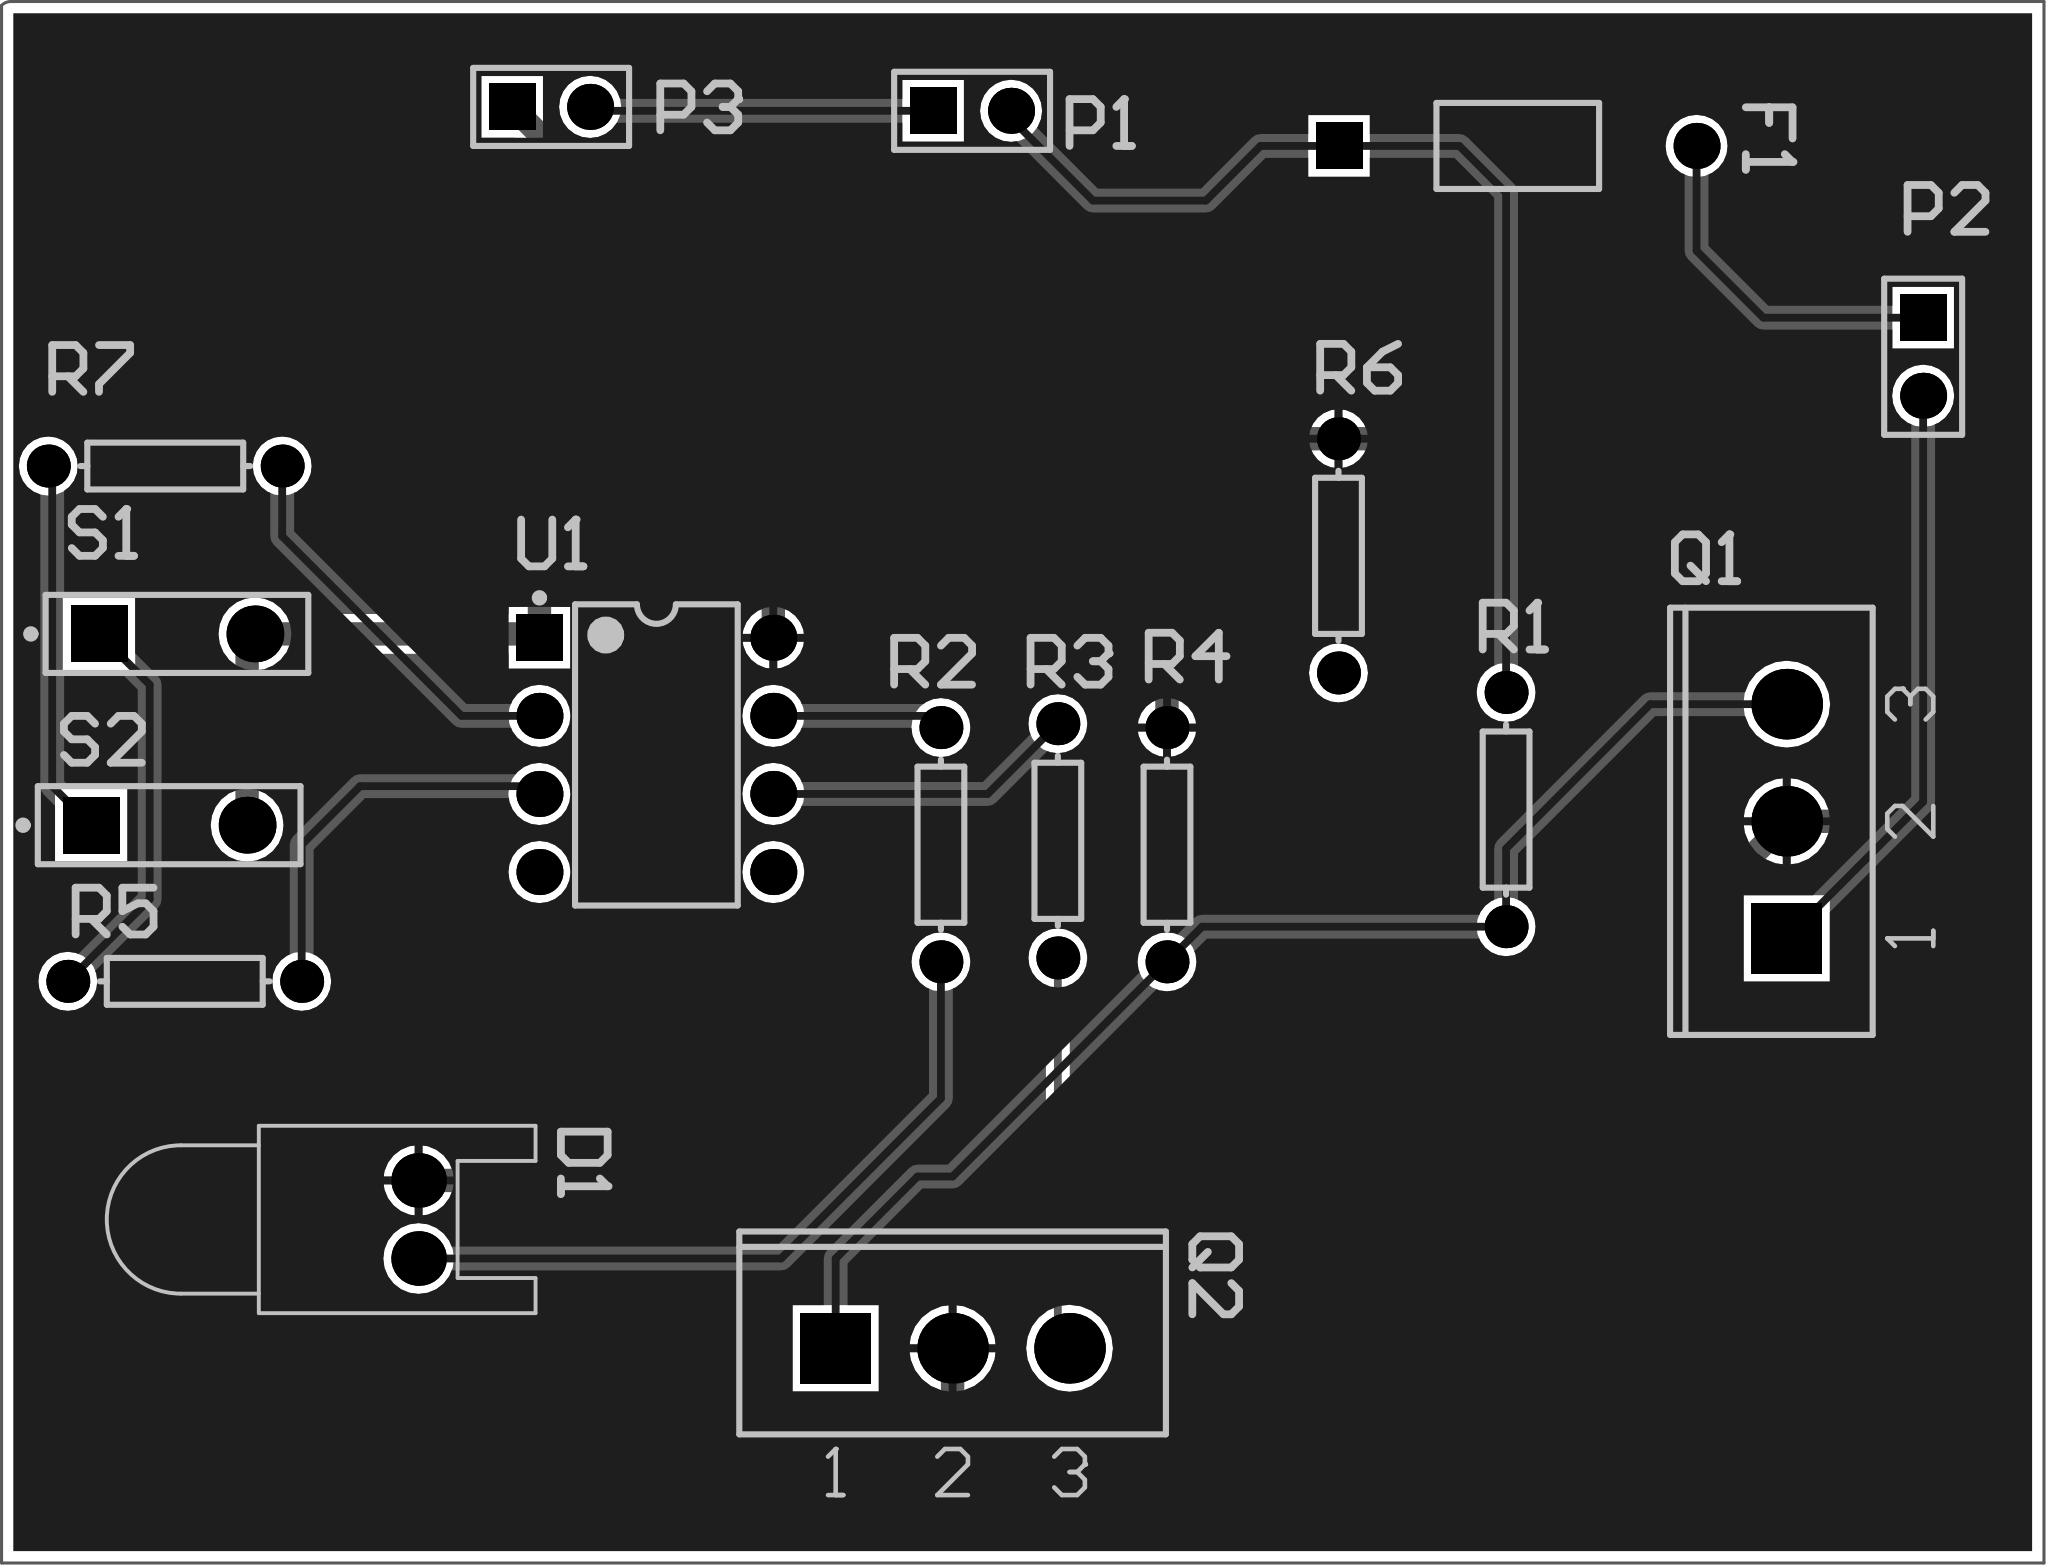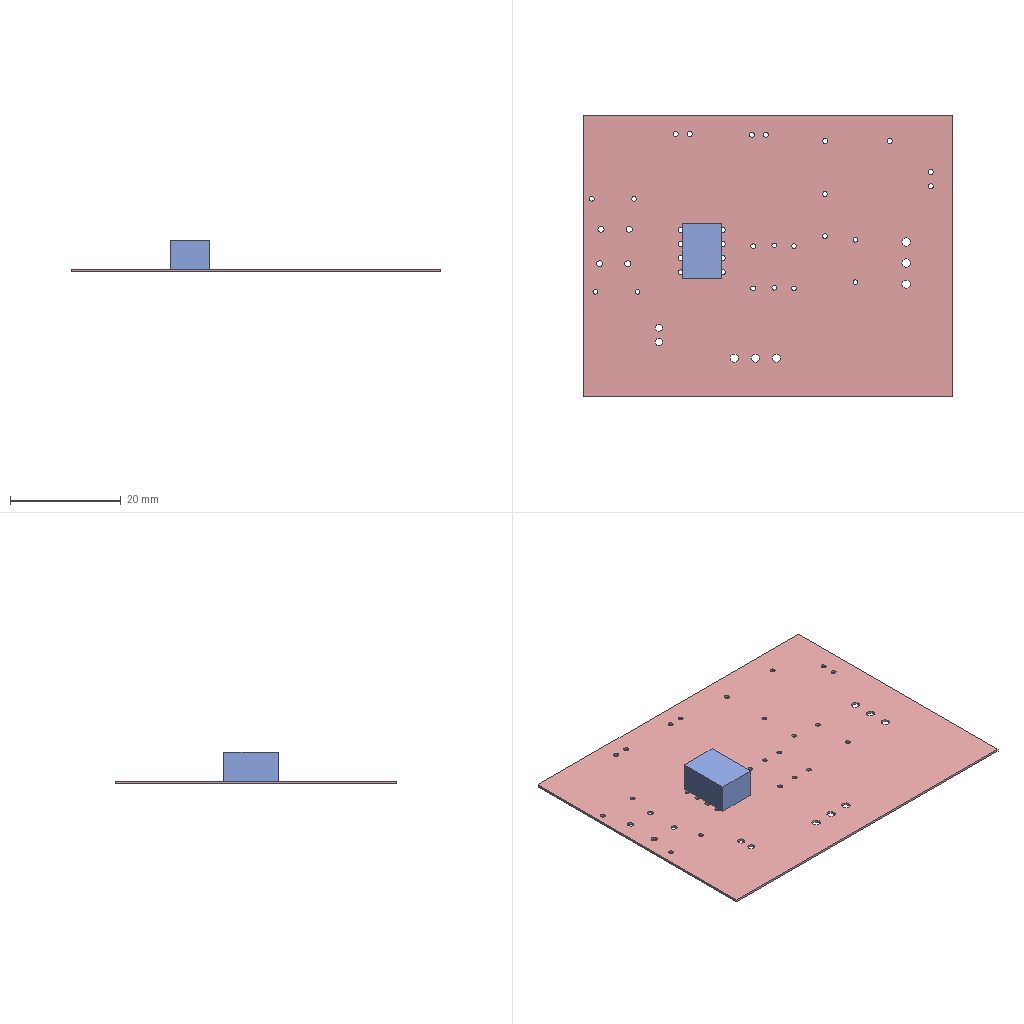Circuit board layout | Altium Designer | box 66.5 x 50.8 x 5.8 mm
Layer stack:
# Altium Designer layer stack of  (unit mm; dielectric type: 0 none, 1 core, 2 prepreg, 3 surface material)
index,name,kind,layer,copper_thickness_mm,dielectric_type,dielectric_thickness_mm,dielectric_material,dielectric_constant
0,Top Paste,other,,,,,,
1,Top Overlay,other,,,,,,
2,Top Solder,dielectric,,,3,0.0102,Solder Resist,3.5
3,Top Layer,copper,Top Layer,0.0356,,,,
4,Dielectric 1,dielectric,,,0,0.32,FR-4,4.8
5,Bottom Layer,copper,Bottom Layer,0.0356,,,,
6,Bottom Solder,dielectric,,,3,0.0102,Solder Resist,3.5
7,Bottom Overlay,other,,,,,,
8,Bottom Paste,other,,,,,,
# drill layer pairs: low layer,high layer
drill_pair,Top Layer,Bottom Layer
Part placement:
Designator,Comment,Layer,Footprint,Center-X(mm),Center-Y(mm),Rotation
U1,PIC12F508-E/P,TopLayer,PDIP300-P8,91.313,56.134,0
S2,SW-SPST,TopLayer,SPST-2,75.438,53.848,360
S1,SW-SPST,TopLayer,SPST-2,75.692,60.071,360
R7,10K,TopLayer,AXIAL-0.3,75.311,65.532,180
R6,10K,TopLayer,AXIAL-0.3,113.538,62.611,90
R5,10K,TopLayer,AXIAL-0.3,75.946,48.768,180
R4,47K,TopLayer,AXIAL-0.3,107.95,53.213,90
R3,100,TopLayer,AXIAL-0.3,104.394,53.34,270
R2,150,TopLayer,AXIAL-0.3,100.584,53.213,270
R1,220,TopLayer,AXIAL-0.3,118.999,54.356,270
Q2,JANTXV2N7224,TopLayer,TO-254AA,100.965,36.83,360
Q1,JANTXV2N7224,TopLayer,TO-254AA,128.143,53.975,90
P3,5VINPUT,TopLayer,HDR1X2,87.884,77.216,360
P2,POW OUTPUT,TopLayer,HDR1X2,132.588,69.088,270
P1,24VINPUT,TopLayer,HDR1X2,101.6,77.089,360
F1,24V,TopLayer,PIN-W2/E2.8,119.38,75.946,360
D1,LED0,TopLayer,LED-0,83.566,41.021,270
Pad and via stacks:
# Altium Designer via and pad stacks of  (unit mm). Each distinct definition once, with the count of objects using it.
# via: kind,start_layer,end_layer,hole_mm,diameter_mm,mode(0 simple;1 top-mid-bottom;2 full stack),diameter_per_layer,count,example_net
# pad: kind,layer,hole_mm,hole_type(0 round;1 square;2 slot),plating,top_size,top_shape(1 round;2 rect;3 octagon;9 rounded rect),mid_size,bottom_size,mode,footprint,size_per_layer,count,example
pad,Multi-Layer,0.9,0,plated,1.5x1.5,2,1.5x1.5,1.5x1.5,0,HDR1X2,,3,P2.1
pad,Multi-Layer,0.9,0,plated,1.5x1.5,1,1.5x1.5,1.5x1.5,0,HDR1X2,,3,P2.2
pad,Multi-Layer,0.9,0,plated,1.5x1.5,1,1.5x1.5,1.5x1.5,0,PIN-W2/E2.8,,1,F1.2
pad,Multi-Layer,0.9,0,plated,1.5x1.5,2,1.5x1.5,1.5x1.5,0,PIN-W2/E2.8,,1,F1.1
pad,Multi-Layer,0.85,0,plated,1.4x1.4,1,1.4x1.4,1.4x1.4,0,AXIAL-0.3,,14,R1.2
pad,Multi-Layer,1.27,0,plated,1.778x1.778,1,1.778x1.778,1.778x1.778,0,LED-0,,2,D1.1
pad,Multi-Layer,1.5,0,plated,2.3x2.3,2,2.3x2.3,2.3x2.3,0,TO-254AA,,2,Q1.1
pad,Multi-Layer,1.5,0,plated,2.3x2.3,1,2.3x2.3,2.3x2.3,0,TO-254AA,,4,Q1.2
pad,Multi-Layer,0.9,0,plated,1.5x1.5,1,1.5x1.5,1.5x1.5,0,PDIP300-P8,,7,U1.5
pad,Multi-Layer,0.9,0,plated,1.5x1.5,2,1.5x1.5,1.5x1.5,0,PDIP300-P8,,1,U1.1
pad,Multi-Layer,1.1,0,plated,1.85x1.85,2,1.85x1.85,1.85x1.85,0,SPST-2,,2,S1.1
pad,Multi-Layer,1.1,0,plated,1.85x1.85,1,1.85x1.85,1.85x1.85,0,SPST-2,,2,S1.2
Copper pours:
name,layer,net,type(0 solid;1 hatched;2 none)
D,Bottom Layer,GND,0
D,Top Layer,GND,0
Design rules, without the lines most boards share:
# Altium Designer design rules of  (exported by Altium Designer, unit mm)
# columns: name | kind | enabled | priority | scope1 | scope2 | descriptor | typed fields (field=value)
SilkToSilkClearance | 55 | enabled | 1 | All | All | Silk to Silk (Clearance=0mil) (All),(All) |
SilkToSolderMaskClearance | 54 | enabled | 1 | IsPad | All | Silk To Solder Mask (Clearance=0mil) (IsPad),(All) |
MinimumSolderMaskSliver | 53 | enabled | 1 | All | All | Minimum Solder Mask Sliver (Gap=0mil) (All),(All) |
HoleToHoleClearance | 52 | enabled | 1 | All | All | Hole To Hole Clearance (Gap=10mil) (All),(All) | gap=0.254
DiffPairsRouting | 51 | enabled | 1 | All | All | Differential Pairs Uncoupled Length using the Gap Constraints (Min=10mil) (Max=10mil) (Prefered=10mil)  and Width Constraints (Min=15mil) (Max=15mil) (Prefered=15mil) (All) |
SolderMaskExpansion | 13 | enabled | 1 | All | All | Solder Mask Expansion (Expansion =4mil) (All) | expansion=0.1016
PasteMaskExpansion | 14 | enabled | 1 | All | All | Paste Mask Expansion (Expansion =0mil) (All) | expansion=0
RoutingVias | 11 | enabled | 1 | All | All | Routing Via (MinHoleWidth=28mil) (MaxHoleWidth=28mil) (PreferredHoleWidth=28mil) (MinWidth=50mil) (MaxWidth=50mil) (PreferedWidth=50mil) (All) | via_min_hole=0.7112 via_max_hole=0.7112 via_preferred_diameter=1.27 via_preferred_hole=0.7112
Width | 2 | enabled | 1 | All | All | Width Constraint (Min=10mil) (Max=30mil) (Preferred=10mil) (All) |
PolygonConnect | 20 | enabled | 1 | All | All | Polygon Connect Rule(Relief Connect )(Conductor Width=10mil) (Relief Angle=90 Angle) (Entries=4) (Air Gap Width=10mil) (All),(All) | connect_style(0=relief,1=direct,2=none)=0 relief_conductor_width=0.254 relief_entries=4
PlaneConnect | 6 | enabled | 1 | All | All | Power Plane Connect Rule(Relief Connect )(Expansion=20mil) (Conductor Width=10mil) (Air Gap=10mil) (Entries=4) (All) | relief_conductor_width=0.254 relief_entries=4 relief_expansion=0.508
Clearance | 0 | enabled | 1 | All | All | Clearance Constraint (Gap=10mil) (All),(All) | gap=0.254
Classes set for this board:
# Altium Designer classes of  (member kind: 0 net, 1 component, 2 from-to, 3 pad, 4 layer, 5 differential pair, 6 design channel, 7 polygon, 8 structure, 9 xSignal)
# columns: class name | member kind | superclass | members
Sheet1 | 1 | no | D1; F1; P1; P2; P3; Q1; Q2; R1; R2; R3; R4; R5; R6; R7; S1; S2; U1;